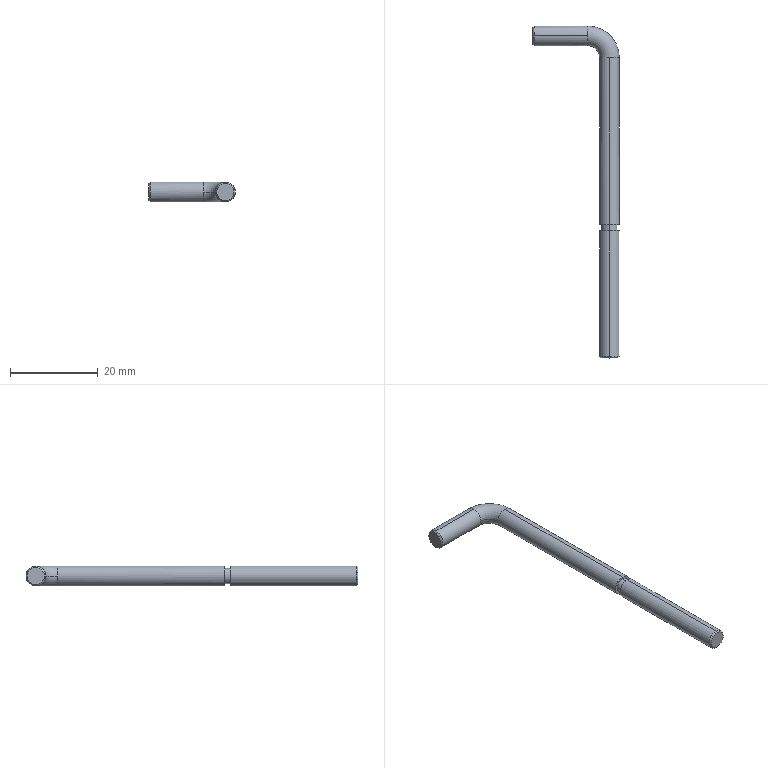Part | SolidWorks | features Chamfer 1, RevCut 1, Sweep 1 | 1 solid | 18 faces | box 19.75 x 75.75 x 4.5 mm | volume 1403 mm3 | cylinder 8 | cone 4 | plane 4 | torus 2 | commonest cylinder face diameters 4.5 x6 3.5 x2
STEP:
#1=CARTESIAN_POINT('',(0.,68.5,2.25));
#2=VERTEX_POINT('',#1);
#3=CARTESIAN_POINT('',(2.25,68.5,0.));
#4=VERTEX_POINT('',#3);
#5=CARTESIAN_POINT('',(0.,68.5,0.));
#6=DIRECTION('',(0.,1.,0.));
#7=DIRECTION('',(0.,0.,1.));
#8=AXIS2_PLACEMENT_3D('',#5,#6,#7);
#9=CIRCLE('',#8,2.25);
#10=EDGE_CURVE('',#2,#4,#9,.T.);
#11=ORIENTED_EDGE('',*,*,#10,.T.);
#12=CARTESIAN_POINT('',(-5.,75.75,0.));
#13=VERTEX_POINT('',#12);
#14=CARTESIAN_POINT('',(-5.,68.5,0.));
#15=DIRECTION('',(0.,0.,1.));
#16=DIRECTION('',(1.,0.,0.));
#17=AXIS2_PLACEMENT_3D('',#14,#15,#16);
#18=CIRCLE('',#17,7.25);
#19=EDGE_CURVE('',#4,#13,#18,.T.);
#20=ORIENTED_EDGE('',*,*,#19,.T.);
#21=CARTESIAN_POINT('',(-5.,73.5,2.25));
#22=VERTEX_POINT('',#21);
#23=CARTESIAN_POINT('',(-5.,73.5,0.));
#24=DIRECTION('',(-1.,0.,0.));
#25=DIRECTION('',(0.,0.,1.));
#26=AXIS2_PLACEMENT_3D('',#23,#24,#25);
#27=CIRCLE('',#26,2.25);
#28=EDGE_CURVE('',#22,#13,#27,.T.);
#29=ORIENTED_EDGE('',*,*,#28,.F.);
#30=CARTESIAN_POINT('',(-5.,71.25,0.));
#31=VERTEX_POINT('',#30);
#32=CARTESIAN_POINT('',(-5.,73.5,0.));
#33=DIRECTION('',(-1.,0.,0.));
#34=DIRECTION('',(0.,0.,1.));
#35=AXIS2_PLACEMENT_3D('',#32,#33,#34);
#36=CIRCLE('',#35,2.25);
#37=EDGE_CURVE('',#31,#22,#36,.T.);
#38=ORIENTED_EDGE('',*,*,#37,.F.);
#39=CARTESIAN_POINT('',(-2.25,68.5,0.));
#40=VERTEX_POINT('',#39);
#41=CARTESIAN_POINT('',(-5.,68.5,0.));
#42=DIRECTION('',(0.,0.,1.));
#43=DIRECTION('',(1.,0.,0.));
#44=AXIS2_PLACEMENT_3D('',#41,#42,#43);
#45=CIRCLE('',#44,2.75);
#46=EDGE_CURVE('',#40,#31,#45,.T.);
#47=ORIENTED_EDGE('',*,*,#46,.F.);
#48=CARTESIAN_POINT('',(0.,68.5,0.));
#49=DIRECTION('',(0.,1.,0.));
#50=DIRECTION('',(0.,0.,1.));
#51=AXIS2_PLACEMENT_3D('',#48,#49,#50);
#52=CIRCLE('',#51,2.25);
#53=EDGE_CURVE('',#40,#2,#52,.T.);
#54=ORIENTED_EDGE('',*,*,#53,.T.);
#55=EDGE_LOOP('',(#11,#20,#29,#38,#47,#54));
#56=FACE_OUTER_BOUND('',#55,.T.);
#57=CARTESIAN_POINT('',(-5.,68.5,0.));
#58=DIRECTION('',(0.,0.,1.));
#59=DIRECTION('',(1.,0.,0.));
#60=AXIS2_PLACEMENT_3D('',#57,#58,#59);
#61=TOROIDAL_SURFACE('',#60,5.,2.25);
#62=ADVANCED_FACE('',(#56),#61,.T.);
#63=CARTESIAN_POINT('',(0.,0.,-1.95));
#64=VERTEX_POINT('',#63);
#65=CARTESIAN_POINT('',(0.,0.,1.95));
#66=VERTEX_POINT('',#65);
#67=CARTESIAN_POINT('',(0.,0.,0.));
#68=DIRECTION('',(0.,-1.,0.));
#69=DIRECTION('',(0.,0.,1.));
#70=AXIS2_PLACEMENT_3D('',#67,#68,#69);
#71=CIRCLE('',#70,1.95);
#72=EDGE_CURVE('',#64,#66,#71,.T.);
#73=ORIENTED_EDGE('',*,*,#72,.F.);
#74=CARTESIAN_POINT('',(0.,0.3,-2.25));
#75=VERTEX_POINT('',#74);
#76=CARTESIAN_POINT('',(0.,0.3,-2.25));
#77=DIRECTION('',(0.,0.7071,-0.7071));
#78=VECTOR('',#77,1000.);
#79=LINE('',#76,#78);
#80=EDGE_CURVE('',#64,#75,#79,.T.);
#81=ORIENTED_EDGE('',*,*,#80,.T.);
#82=CARTESIAN_POINT('',(0.,0.3,2.25));
#83=VERTEX_POINT('',#82);
#84=CARTESIAN_POINT('',(0.,0.3,0.));
#85=DIRECTION('',(0.,1.,0.));
#86=DIRECTION('',(0.,0.,1.));
#87=AXIS2_PLACEMENT_3D('',#84,#85,#86);
#88=CIRCLE('',#87,2.25);
#89=EDGE_CURVE('',#83,#75,#88,.T.);
#90=ORIENTED_EDGE('',*,*,#89,.F.);
#91=CARTESIAN_POINT('',(0.,0.3,2.25));
#92=DIRECTION('',(0.,0.7071,0.7071));
#93=VECTOR('',#92,1000.);
#94=LINE('',#91,#93);
#95=EDGE_CURVE('',#66,#83,#94,.T.);
#96=ORIENTED_EDGE('',*,*,#95,.F.);
#97=EDGE_LOOP('',(#73,#81,#90,#96));
#98=FACE_OUTER_BOUND('',#97,.T.);
#99=CARTESIAN_POINT('',(0.,0.3,0.));
#100=DIRECTION('',(0.,1.,0.));
#101=DIRECTION('',(0.,0.,1.));
#102=AXIS2_PLACEMENT_3D('',#99,#100,#101);
#103=CONICAL_SURFACE('',#102,2.25,0.7854);
#104=ADVANCED_FACE('',(#98),#103,.T.);
#105=CARTESIAN_POINT('',(-17.5,73.5,1.95));
#106=VERTEX_POINT('',#105);
#107=CARTESIAN_POINT('',(-17.5,73.5,-1.95));
#108=VERTEX_POINT('',#107);
#109=CARTESIAN_POINT('',(-17.5,73.5,0.));
#110=DIRECTION('',(-1.,0.,0.));
#111=DIRECTION('',(0.,-1.,0.));
#112=AXIS2_PLACEMENT_3D('',#109,#110,#111);
#113=CIRCLE('',#112,1.95);
#114=EDGE_CURVE('',#106,#108,#113,.T.);
#115=ORIENTED_EDGE('',*,*,#114,.F.);
#116=CARTESIAN_POINT('',(-17.2,73.5,2.25));
#117=VERTEX_POINT('',#116);
#118=CARTESIAN_POINT('',(-17.5,73.5,1.95));
#119=DIRECTION('',(0.7071,0.,0.7071));
#120=VECTOR('',#119,1000.);
#121=LINE('',#118,#120);
#122=EDGE_CURVE('',#106,#117,#121,.T.);
#123=ORIENTED_EDGE('',*,*,#122,.T.);
#124=CARTESIAN_POINT('',(-17.2,73.5,-2.25));
#125=VERTEX_POINT('',#124);
#126=CARTESIAN_POINT('',(-17.2,73.5,0.));
#127=DIRECTION('',(1.,0.,0.));
#128=DIRECTION('',(0.,0.,1.));
#129=AXIS2_PLACEMENT_3D('',#126,#127,#128);
#130=CIRCLE('',#129,2.25);
#131=EDGE_CURVE('',#125,#117,#130,.T.);
#132=ORIENTED_EDGE('',*,*,#131,.F.);
#133=CARTESIAN_POINT('',(-17.5,73.5,-1.95));
#134=DIRECTION('',(0.7071,0.,-0.7071));
#135=VECTOR('',#134,1000.);
#136=LINE('',#133,#135);
#137=EDGE_CURVE('',#108,#125,#136,.T.);
#138=ORIENTED_EDGE('',*,*,#137,.F.);
#139=EDGE_LOOP('',(#115,#123,#132,#138));
#140=FACE_OUTER_BOUND('',#139,.T.);
#141=CARTESIAN_POINT('',(-17.5,73.5,0.));
#142=DIRECTION('',(1.,0.,0.));
#143=DIRECTION('',(0.,0.,-1.));
#144=AXIS2_PLACEMENT_3D('',#141,#142,#143);
#145=CONICAL_SURFACE('',#144,1.95,0.7854);
#146=ADVANCED_FACE('',(#140),#145,.T.);
#147=CARTESIAN_POINT('',(0.,29.,-2.25));
#148=VERTEX_POINT('',#147);
#149=CARTESIAN_POINT('',(0.,29.,2.25));
#150=VERTEX_POINT('',#149);
#151=CARTESIAN_POINT('',(0.,29.,0.));
#152=DIRECTION('',(0.,-1.,0.));
#153=DIRECTION('',(0.,0.,-1.));
#154=AXIS2_PLACEMENT_3D('',#151,#152,#153);
#155=CIRCLE('',#154,2.25);
#156=EDGE_CURVE('',#148,#150,#155,.T.);
#157=ORIENTED_EDGE('',*,*,#156,.T.);
#158=CARTESIAN_POINT('',(0.,68.5,2.25));
#159=DIRECTION('',(0.,-1.,0.));
#160=VECTOR('',#159,1000.);
#161=LINE('',#158,#160);
#162=EDGE_CURVE('',#150,#83,#161,.T.);
#163=ORIENTED_EDGE('',*,*,#162,.T.);
#164=ORIENTED_EDGE('',*,*,#89,.T.);
#165=CARTESIAN_POINT('',(0.,68.5,-2.25));
#166=DIRECTION('',(0.,-1.,0.));
#167=VECTOR('',#166,1000.);
#168=LINE('',#165,#167);
#169=EDGE_CURVE('',#148,#75,#168,.T.);
#170=ORIENTED_EDGE('',*,*,#169,.F.);
#171=EDGE_LOOP('',(#157,#163,#164,#170));
#172=FACE_OUTER_BOUND('',#171,.T.);
#173=CARTESIAN_POINT('',(0.,68.5,0.));
#174=DIRECTION('',(0.,-1.,0.));
#175=DIRECTION('',(0.,0.,-1.));
#176=AXIS2_PLACEMENT_3D('',#173,#174,#175);
#177=CYLINDRICAL_SURFACE('',#176,2.25);
#178=ADVANCED_FACE('',(#172),#177,.T.);
#179=CARTESIAN_POINT('',(0.,30.5,-1.75));
#180=VERTEX_POINT('',#179);
#181=CARTESIAN_POINT('',(0.,30.5,1.75));
#182=VERTEX_POINT('',#181);
#183=CARTESIAN_POINT('',(0.,30.5,0.));
#184=DIRECTION('',(0.,-1.,0.));
#185=DIRECTION('',(0.,0.,-1.));
#186=AXIS2_PLACEMENT_3D('',#183,#184,#185);
#187=CIRCLE('',#186,1.75);
#188=EDGE_CURVE('',#180,#182,#187,.T.);
#189=ORIENTED_EDGE('',*,*,#188,.T.);
#190=CARTESIAN_POINT('',(0.,29.,1.75));
#191=VERTEX_POINT('',#190);
#192=CARTESIAN_POINT('',(0.,0.,1.75));
#193=DIRECTION('',(0.,-1.,0.));
#194=VECTOR('',#193,1000.);
#195=LINE('',#192,#194);
#196=EDGE_CURVE('',#182,#191,#195,.T.);
#197=ORIENTED_EDGE('',*,*,#196,.T.);
#198=CARTESIAN_POINT('',(0.,29.,-1.75));
#199=VERTEX_POINT('',#198);
#200=CARTESIAN_POINT('',(0.,29.,0.));
#201=DIRECTION('',(0.,-1.,0.));
#202=DIRECTION('',(0.,0.,-1.));
#203=AXIS2_PLACEMENT_3D('',#200,#201,#202);
#204=CIRCLE('',#203,1.75);
#205=EDGE_CURVE('',#199,#191,#204,.T.);
#206=ORIENTED_EDGE('',*,*,#205,.F.);
#207=CARTESIAN_POINT('',(0.,0.,-1.75));
#208=DIRECTION('',(0.,-1.,0.));
#209=VECTOR('',#208,1000.);
#210=LINE('',#207,#209);
#211=EDGE_CURVE('',#180,#199,#210,.T.);
#212=ORIENTED_EDGE('',*,*,#211,.F.);
#213=EDGE_LOOP('',(#189,#197,#206,#212));
#214=FACE_OUTER_BOUND('',#213,.T.);
#215=CARTESIAN_POINT('',(0.,0.,0.));
#216=DIRECTION('',(0.,-1.,0.));
#217=DIRECTION('',(0.,0.,-1.));
#218=AXIS2_PLACEMENT_3D('',#215,#216,#217);
#219=CYLINDRICAL_SURFACE('',#218,1.75);
#220=ADVANCED_FACE('',(#214),#219,.T.);
#221=ORIENTED_EDGE('',*,*,#10,.F.);
#222=CARTESIAN_POINT('',(0.,30.5,2.25));
#223=VERTEX_POINT('',#222);
#224=CARTESIAN_POINT('',(0.,68.5,2.25));
#225=DIRECTION('',(0.,-1.,0.));
#226=VECTOR('',#225,1000.);
#227=LINE('',#224,#226);
#228=EDGE_CURVE('',#2,#223,#227,.T.);
#229=ORIENTED_EDGE('',*,*,#228,.T.);
#230=CARTESIAN_POINT('',(0.,30.5,-2.25));
#231=VERTEX_POINT('',#230);
#232=CARTESIAN_POINT('',(0.,30.5,0.));
#233=DIRECTION('',(0.,-1.,0.));
#234=DIRECTION('',(0.,0.,-1.));
#235=AXIS2_PLACEMENT_3D('',#232,#233,#234);
#236=CIRCLE('',#235,2.25);
#237=EDGE_CURVE('',#231,#223,#236,.T.);
#238=ORIENTED_EDGE('',*,*,#237,.F.);
#239=CARTESIAN_POINT('',(0.,68.5,-2.25));
#240=VERTEX_POINT('',#239);
#241=CARTESIAN_POINT('',(0.,68.5,-2.25));
#242=DIRECTION('',(0.,-1.,0.));
#243=VECTOR('',#242,1000.);
#244=LINE('',#241,#243);
#245=EDGE_CURVE('',#240,#231,#244,.T.);
#246=ORIENTED_EDGE('',*,*,#245,.F.);
#247=CARTESIAN_POINT('',(0.,68.5,0.));
#248=DIRECTION('',(0.,1.,0.));
#249=DIRECTION('',(0.,0.,1.));
#250=AXIS2_PLACEMENT_3D('',#247,#248,#249);
#251=CIRCLE('',#250,2.25);
#252=EDGE_CURVE('',#4,#240,#251,.T.);
#253=ORIENTED_EDGE('',*,*,#252,.F.);
#254=EDGE_LOOP('',(#221,#229,#238,#246,#253));
#255=FACE_OUTER_BOUND('',#254,.T.);
#256=CARTESIAN_POINT('',(0.,68.5,0.));
#257=DIRECTION('',(0.,-1.,0.));
#258=DIRECTION('',(0.,0.,-1.));
#259=AXIS2_PLACEMENT_3D('',#256,#257,#258);
#260=CYLINDRICAL_SURFACE('',#259,2.25);
#261=ADVANCED_FACE('',(#255),#260,.T.);
#262=ORIENTED_EDGE('',*,*,#28,.T.);
#263=CARTESIAN_POINT('',(-5.,73.5,-2.25));
#264=VERTEX_POINT('',#263);
#265=CARTESIAN_POINT('',(-5.,73.5,0.));
#266=DIRECTION('',(-1.,0.,0.));
#267=DIRECTION('',(0.,0.,1.));
#268=AXIS2_PLACEMENT_3D('',#265,#266,#267);
#269=CIRCLE('',#268,2.25);
#270=EDGE_CURVE('',#13,#264,#269,.T.);
#271=ORIENTED_EDGE('',*,*,#270,.T.);
#272=CARTESIAN_POINT('',(-5.,73.5,-2.25));
#273=DIRECTION('',(-1.,0.,0.));
#274=VECTOR('',#273,1000.);
#275=LINE('',#272,#274);
#276=EDGE_CURVE('',#264,#125,#275,.T.);
#277=ORIENTED_EDGE('',*,*,#276,.T.);
#278=ORIENTED_EDGE('',*,*,#131,.T.);
#279=CARTESIAN_POINT('',(-5.,73.5,2.25));
#280=DIRECTION('',(-1.,0.,0.));
#281=VECTOR('',#280,1000.);
#282=LINE('',#279,#281);
#283=EDGE_CURVE('',#22,#117,#282,.T.);
#284=ORIENTED_EDGE('',*,*,#283,.F.);
#285=EDGE_LOOP('',(#262,#271,#277,#278,#284));
#286=FACE_OUTER_BOUND('',#285,.T.);
#287=CARTESIAN_POINT('',(-5.,73.5,0.));
#288=DIRECTION('',(-1.,0.,0.));
#289=DIRECTION('',(0.,0.,1.));
#290=AXIS2_PLACEMENT_3D('',#287,#288,#289);
#291=CYLINDRICAL_SURFACE('',#290,2.25);
#292=ADVANCED_FACE('',(#286),#291,.T.);
#293=ORIENTED_EDGE('',*,*,#276,.F.);
#294=CARTESIAN_POINT('',(-5.,73.5,0.));
#295=DIRECTION('',(-1.,0.,0.));
#296=DIRECTION('',(0.,0.,1.));
#297=AXIS2_PLACEMENT_3D('',#294,#295,#296);
#298=CIRCLE('',#297,2.25);
#299=EDGE_CURVE('',#264,#31,#298,.T.);
#300=ORIENTED_EDGE('',*,*,#299,.T.);
#301=ORIENTED_EDGE('',*,*,#37,.T.);
#302=ORIENTED_EDGE('',*,*,#283,.T.);
#303=CARTESIAN_POINT('',(-17.2,73.5,0.));
#304=DIRECTION('',(1.,0.,0.));
#305=DIRECTION('',(0.,0.,1.));
#306=AXIS2_PLACEMENT_3D('',#303,#304,#305);
#307=CIRCLE('',#306,2.25);
#308=EDGE_CURVE('',#117,#125,#307,.T.);
#309=ORIENTED_EDGE('',*,*,#308,.T.);
#310=EDGE_LOOP('',(#293,#300,#301,#302,#309));
#311=FACE_OUTER_BOUND('',#310,.T.);
#312=CARTESIAN_POINT('',(-5.,73.5,0.));
#313=DIRECTION('',(-1.,0.,0.));
#314=DIRECTION('',(0.,0.,1.));
#315=AXIS2_PLACEMENT_3D('',#312,#313,#314);
#316=CYLINDRICAL_SURFACE('',#315,2.25);
#317=ADVANCED_FACE('',(#311),#316,.T.);
#318=ORIENTED_EDGE('',*,*,#19,.F.);
#319=ORIENTED_EDGE('',*,*,#252,.T.);
#320=CARTESIAN_POINT('',(0.,68.5,0.));
#321=DIRECTION('',(0.,1.,0.));
#322=DIRECTION('',(0.,0.,1.));
#323=AXIS2_PLACEMENT_3D('',#320,#321,#322);
#324=CIRCLE('',#323,2.25);
#325=EDGE_CURVE('',#240,#40,#324,.T.);
#326=ORIENTED_EDGE('',*,*,#325,.T.);
#327=ORIENTED_EDGE('',*,*,#46,.T.);
#328=ORIENTED_EDGE('',*,*,#299,.F.);
#329=ORIENTED_EDGE('',*,*,#270,.F.);
#330=EDGE_LOOP('',(#318,#319,#326,#327,#328,#329));
#331=FACE_OUTER_BOUND('',#330,.T.);
#332=CARTESIAN_POINT('',(-5.,68.5,0.));
#333=DIRECTION('',(0.,0.,1.));
#334=DIRECTION('',(1.,0.,0.));
#335=AXIS2_PLACEMENT_3D('',#332,#333,#334);
#336=TOROIDAL_SURFACE('',#335,5.,2.25);
#337=ADVANCED_FACE('',(#331),#336,.T.);
#338=ORIENTED_EDGE('',*,*,#228,.F.);
#339=ORIENTED_EDGE('',*,*,#53,.F.);
#340=ORIENTED_EDGE('',*,*,#325,.F.);
#341=ORIENTED_EDGE('',*,*,#245,.T.);
#342=CARTESIAN_POINT('',(0.,30.5,0.));
#343=DIRECTION('',(0.,-1.,0.));
#344=DIRECTION('',(0.,0.,-1.));
#345=AXIS2_PLACEMENT_3D('',#342,#343,#344);
#346=CIRCLE('',#345,2.25);
#347=EDGE_CURVE('',#223,#231,#346,.T.);
#348=ORIENTED_EDGE('',*,*,#347,.F.);
#349=EDGE_LOOP('',(#338,#339,#340,#341,#348));
#350=FACE_OUTER_BOUND('',#349,.T.);
#351=CARTESIAN_POINT('',(0.,68.5,0.));
#352=DIRECTION('',(0.,-1.,0.));
#353=DIRECTION('',(0.,0.,-1.));
#354=AXIS2_PLACEMENT_3D('',#351,#352,#353);
#355=CYLINDRICAL_SURFACE('',#354,2.25);
#356=ADVANCED_FACE('',(#350),#355,.T.);
#357=CARTESIAN_POINT('',(-17.5,73.5,0.));
#358=DIRECTION('',(-1.,0.,0.));
#359=DIRECTION('',(0.,-1.,0.));
#360=AXIS2_PLACEMENT_3D('',#357,#358,#359);
#361=CIRCLE('',#360,1.95);
#362=EDGE_CURVE('',#108,#106,#361,.T.);
#363=ORIENTED_EDGE('',*,*,#362,.T.);
#364=ORIENTED_EDGE('',*,*,#114,.T.);
#365=EDGE_LOOP('',(#363,#364));
#366=FACE_OUTER_BOUND('',#365,.T.);
#367=CARTESIAN_POINT('',(-17.5,73.5,0.));
#368=DIRECTION('',(-1.,0.,0.));
#369=DIRECTION('',(0.,0.,1.));
#370=AXIS2_PLACEMENT_3D('',#367,#368,#369);
#371=PLANE('',#370);
#372=ADVANCED_FACE('',(#366),#371,.T.);
#373=ORIENTED_EDGE('',*,*,#156,.F.);
#374=CARTESIAN_POINT('',(0.,29.,0.));
#375=DIRECTION('',(0.,-1.,0.));
#376=DIRECTION('',(0.,0.,-1.));
#377=AXIS2_PLACEMENT_3D('',#374,#375,#376);
#378=CIRCLE('',#377,2.25);
#379=EDGE_CURVE('',#150,#148,#378,.T.);
#380=ORIENTED_EDGE('',*,*,#379,.F.);
#381=EDGE_LOOP('',(#373,#380));
#382=FACE_OUTER_BOUND('',#381,.T.);
#383=ORIENTED_EDGE('',*,*,#205,.T.);
#384=CARTESIAN_POINT('',(0.,29.,0.));
#385=DIRECTION('',(0.,-1.,0.));
#386=DIRECTION('',(0.,0.,-1.));
#387=AXIS2_PLACEMENT_3D('',#384,#385,#386);
#388=CIRCLE('',#387,1.75);
#389=EDGE_CURVE('',#191,#199,#388,.T.);
#390=ORIENTED_EDGE('',*,*,#389,.T.);
#391=EDGE_LOOP('',(#383,#390));
#392=FACE_BOUND('',#391,.T.);
#393=CARTESIAN_POINT('',(0.,29.,-1.75));
#394=DIRECTION('',(0.,-1.,0.));
#395=DIRECTION('',(0.,0.,-1.));
#396=AXIS2_PLACEMENT_3D('',#393,#394,#395);
#397=PLANE('',#396);
#398=ADVANCED_FACE('',(#382,#392),#397,.F.);
#399=ORIENTED_EDGE('',*,*,#196,.F.);
#400=CARTESIAN_POINT('',(0.,30.5,0.));
#401=DIRECTION('',(0.,-1.,0.));
#402=DIRECTION('',(0.,0.,-1.));
#403=AXIS2_PLACEMENT_3D('',#400,#401,#402);
#404=CIRCLE('',#403,1.75);
#405=EDGE_CURVE('',#182,#180,#404,.T.);
#406=ORIENTED_EDGE('',*,*,#405,.T.);
#407=ORIENTED_EDGE('',*,*,#211,.T.);
#408=ORIENTED_EDGE('',*,*,#389,.F.);
#409=EDGE_LOOP('',(#399,#406,#407,#408));
#410=FACE_OUTER_BOUND('',#409,.T.);
#411=CARTESIAN_POINT('',(0.,0.,0.));
#412=DIRECTION('',(0.,-1.,0.));
#413=DIRECTION('',(0.,0.,-1.));
#414=AXIS2_PLACEMENT_3D('',#411,#412,#413);
#415=CYLINDRICAL_SURFACE('',#414,1.75);
#416=ADVANCED_FACE('',(#410),#415,.T.);
#417=ORIENTED_EDGE('',*,*,#188,.F.);
#418=ORIENTED_EDGE('',*,*,#405,.F.);
#419=EDGE_LOOP('',(#417,#418));
#420=FACE_BOUND('',#419,.T.);
#421=ORIENTED_EDGE('',*,*,#237,.T.);
#422=ORIENTED_EDGE('',*,*,#347,.T.);
#423=EDGE_LOOP('',(#421,#422));
#424=FACE_OUTER_BOUND('',#423,.T.);
#425=CARTESIAN_POINT('',(0.,30.5,-1.75));
#426=DIRECTION('',(0.,1.,0.));
#427=DIRECTION('',(0.,0.,1.));
#428=AXIS2_PLACEMENT_3D('',#425,#426,#427);
#429=PLANE('',#428);
#430=ADVANCED_FACE('',(#420,#424),#429,.F.);
#431=CARTESIAN_POINT('',(0.,0.,0.));
#432=DIRECTION('',(0.,-1.,0.));
#433=DIRECTION('',(0.,0.,1.));
#434=AXIS2_PLACEMENT_3D('',#431,#432,#433);
#435=CIRCLE('',#434,1.95);
#436=EDGE_CURVE('',#66,#64,#435,.T.);
#437=ORIENTED_EDGE('',*,*,#436,.T.);
#438=ORIENTED_EDGE('',*,*,#72,.T.);
#439=EDGE_LOOP('',(#437,#438));
#440=FACE_OUTER_BOUND('',#439,.T.);
#441=CARTESIAN_POINT('',(0.,0.,0.));
#442=DIRECTION('',(0.,1.,0.));
#443=DIRECTION('',(0.,0.,1.));
#444=AXIS2_PLACEMENT_3D('',#441,#442,#443);
#445=PLANE('',#444);
#446=ADVANCED_FACE('',(#440),#445,.F.);
#447=ORIENTED_EDGE('',*,*,#162,.F.);
#448=ORIENTED_EDGE('',*,*,#379,.T.);
#449=ORIENTED_EDGE('',*,*,#169,.T.);
#450=CARTESIAN_POINT('',(0.,0.3,0.));
#451=DIRECTION('',(0.,1.,0.));
#452=DIRECTION('',(0.,0.,1.));
#453=AXIS2_PLACEMENT_3D('',#450,#451,#452);
#454=CIRCLE('',#453,2.25);
#455=EDGE_CURVE('',#75,#83,#454,.T.);
#456=ORIENTED_EDGE('',*,*,#455,.T.);
#457=EDGE_LOOP('',(#447,#448,#449,#456));
#458=FACE_OUTER_BOUND('',#457,.T.);
#459=CARTESIAN_POINT('',(0.,68.5,0.));
#460=DIRECTION('',(0.,-1.,0.));
#461=DIRECTION('',(0.,0.,-1.));
#462=AXIS2_PLACEMENT_3D('',#459,#460,#461);
#463=CYLINDRICAL_SURFACE('',#462,2.25);
#464=ADVANCED_FACE('',(#458),#463,.T.);
#465=ORIENTED_EDGE('',*,*,#122,.F.);
#466=ORIENTED_EDGE('',*,*,#362,.F.);
#467=ORIENTED_EDGE('',*,*,#137,.T.);
#468=ORIENTED_EDGE('',*,*,#308,.F.);
#469=EDGE_LOOP('',(#465,#466,#467,#468));
#470=FACE_OUTER_BOUND('',#469,.T.);
#471=CARTESIAN_POINT('',(-17.5,73.5,0.));
#472=DIRECTION('',(1.,0.,0.));
#473=DIRECTION('',(0.,0.,-1.));
#474=AXIS2_PLACEMENT_3D('',#471,#472,#473);
#475=CONICAL_SURFACE('',#474,1.95,0.7854);
#476=ADVANCED_FACE('',(#470),#475,.T.);
#477=ORIENTED_EDGE('',*,*,#80,.F.);
#478=ORIENTED_EDGE('',*,*,#436,.F.);
#479=ORIENTED_EDGE('',*,*,#95,.T.);
#480=ORIENTED_EDGE('',*,*,#455,.F.);
#481=EDGE_LOOP('',(#477,#478,#479,#480));
#482=FACE_OUTER_BOUND('',#481,.T.);
#483=CARTESIAN_POINT('',(0.,0.3,0.));
#484=DIRECTION('',(0.,1.,0.));
#485=DIRECTION('',(0.,0.,1.));
#486=AXIS2_PLACEMENT_3D('',#483,#484,#485);
#487=CONICAL_SURFACE('',#486,2.25,0.7854);
#488=ADVANCED_FACE('',(#482),#487,.T.);
#489=CLOSED_SHELL('',(#62,#104,#146,#178,#220,#261,#292,#317,#337,#356,#372,#398,#416,#430,#446,#464,#476,#488));
#490=MANIFOLD_SOLID_BREP('',#489);
#491=CARTESIAN_POINT('',(0.,0.,0.));
#492=DIRECTION('',(0.,0.,1.));
#493=DIRECTION('',(1.,0.,0.));
#494=AXIS2_PLACEMENT_3D('',#491,#492,#493);
#495=(LENGTH_UNIT()NAMED_UNIT(*)SI_UNIT(.MILLI.,.METRE.));
#496=UNCERTAINTY_MEASURE_WITH_UNIT(LENGTH_MEASURE(0.00001),#495,'','');
#497=(NAMED_UNIT(*)PLANE_ANGLE_UNIT()SI_UNIT($,.RADIAN.));
#498=(NAMED_UNIT(*)SI_UNIT($,.STERADIAN.)SOLID_ANGLE_UNIT());
#499=(GEOMETRIC_REPRESENTATION_CONTEXT(3)GLOBAL_UNCERTAINTY_ASSIGNED_CONTEXT((#496))GLOBAL_UNIT_ASSIGNED_CONTEXT((#495,#497,#498))REPRESENTATION_CONTEXT('',''));
#500=ADVANCED_BREP_SHAPE_REPRESENTATION('',(#490,#494),#499);